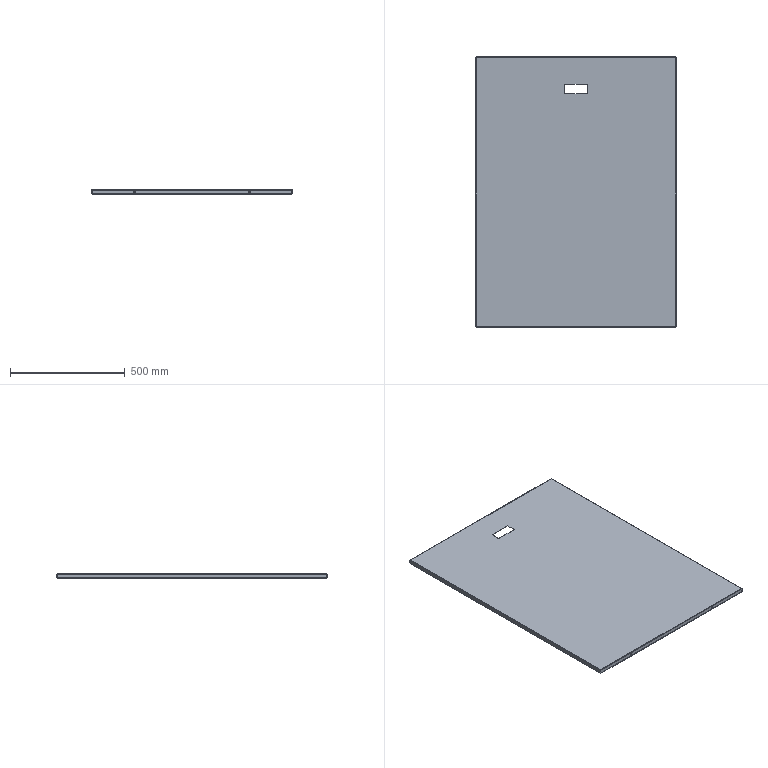Part | SolidWorks | features ICE 6, EdgeFlange 4, CirPattern 2, FlatPattern 1, SMBaseFlange 1, SheetMetal 1 | 1 solid | 109 faces | box 874 x 1178 x 20 mm | volume 1426991 mm3 | plane 63 | cylinder 30 | spline 16 | commonest cylinder face diameters 3 x8 5.4 x8 7.937 x4 9 x4 2 x2 4.4 x2